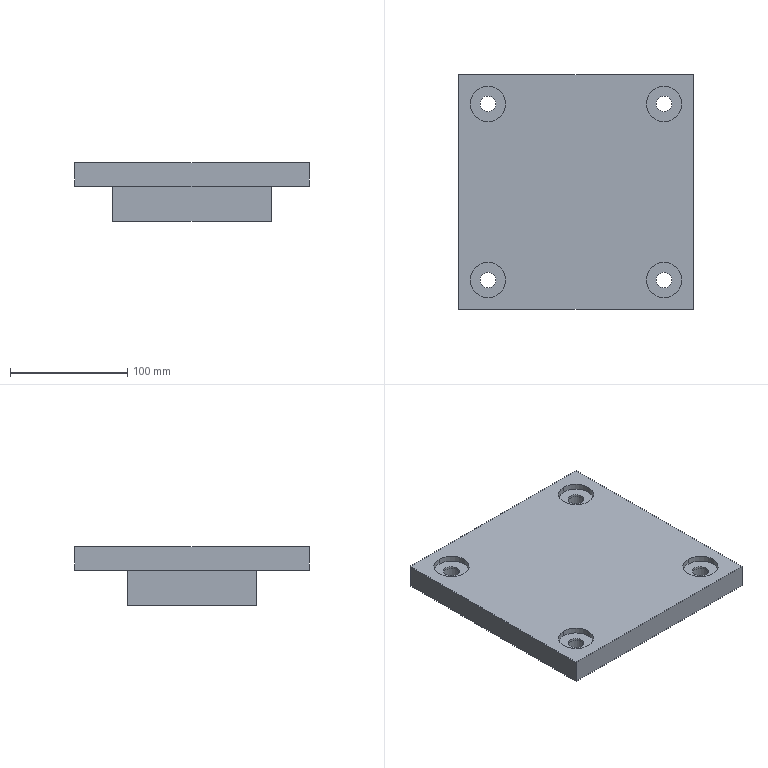Part | SolidWorks | features BaseBody 1 | 1 solid | 43 faces | box 200 x 200 x 50 mm | volume 1213881 mm3 | cylinder 24 | plane 19 | commonest cylinder face diameters 13.5 x8 20 x8 30 x8
STEP:
#1=CARTESIAN_POINT('',(65.,75.,18.));
#2=VERTEX_POINT('',#1);
#3=CARTESIAN_POINT('',(85.,75.,18.));
#4=VERTEX_POINT('',#3);
#5=CARTESIAN_POINT('',(75.,75.,18.));
#6=DIRECTION('',(0.,0.,1.));
#7=DIRECTION('',(-1.,0.,0.));
#8=AXIS2_PLACEMENT_3D('',#5,#6,#7);
#9=CIRCLE('',#8,10.);
#10=EDGE_CURVE('',#2,#4,#9,.T.);
#11=ORIENTED_EDGE('',*,*,#10,.T.);
#12=CARTESIAN_POINT('',(85.,75.,5.));
#13=VERTEX_POINT('',#12);
#14=CARTESIAN_POINT('',(85.,75.,18.));
#15=DIRECTION('',(0.,0.,-1.));
#16=VECTOR('',#15,1000.);
#17=LINE('',#14,#16);
#18=EDGE_CURVE('',#4,#13,#17,.T.);
#19=ORIENTED_EDGE('',*,*,#18,.T.);
#20=CARTESIAN_POINT('',(65.,75.,5.));
#21=VERTEX_POINT('',#20);
#22=CARTESIAN_POINT('',(75.,75.,5.));
#23=DIRECTION('',(0.,0.,-1.));
#24=DIRECTION('',(-1.,0.,0.));
#25=AXIS2_PLACEMENT_3D('',#22,#23,#24);
#26=CIRCLE('',#25,10.);
#27=EDGE_CURVE('',#13,#21,#26,.T.);
#28=ORIENTED_EDGE('',*,*,#27,.T.);
#29=CARTESIAN_POINT('',(65.,75.,18.));
#30=DIRECTION('',(0.,0.,-1.));
#31=VECTOR('',#30,1000.);
#32=LINE('',#29,#31);
#33=EDGE_CURVE('',#2,#21,#32,.T.);
#34=ORIENTED_EDGE('',*,*,#33,.F.);
#35=EDGE_LOOP('',(#11,#19,#28,#34));
#36=FACE_OUTER_BOUND('',#35,.T.);
#37=CARTESIAN_POINT('',(75.,75.,18.));
#38=DIRECTION('',(0.,0.,-1.));
#39=DIRECTION('',(-1.,0.,0.));
#40=AXIS2_PLACEMENT_3D('',#37,#38,#39);
#41=CYLINDRICAL_SURFACE('',#40,10.);
#42=ADVANCED_FACE('',(#36),#41,.F.);
#43=CARTESIAN_POINT('',(-85.,75.,18.));
#44=VERTEX_POINT('',#43);
#45=CARTESIAN_POINT('',(-65.,75.,18.));
#46=VERTEX_POINT('',#45);
#47=CARTESIAN_POINT('',(-75.,75.,18.));
#48=DIRECTION('',(0.,0.,1.));
#49=DIRECTION('',(-1.,0.,0.));
#50=AXIS2_PLACEMENT_3D('',#47,#48,#49);
#51=CIRCLE('',#50,10.);
#52=EDGE_CURVE('',#44,#46,#51,.T.);
#53=ORIENTED_EDGE('',*,*,#52,.T.);
#54=CARTESIAN_POINT('',(-65.,75.,5.));
#55=VERTEX_POINT('',#54);
#56=CARTESIAN_POINT('',(-65.,75.,18.));
#57=DIRECTION('',(0.,0.,-1.));
#58=VECTOR('',#57,1000.);
#59=LINE('',#56,#58);
#60=EDGE_CURVE('',#46,#55,#59,.T.);
#61=ORIENTED_EDGE('',*,*,#60,.T.);
#62=CARTESIAN_POINT('',(-85.,75.,5.));
#63=VERTEX_POINT('',#62);
#64=CARTESIAN_POINT('',(-75.,75.,5.));
#65=DIRECTION('',(0.,0.,1.));
#66=DIRECTION('',(-1.,0.,0.));
#67=AXIS2_PLACEMENT_3D('',#64,#65,#66);
#68=CIRCLE('',#67,10.);
#69=EDGE_CURVE('',#63,#55,#68,.T.);
#70=ORIENTED_EDGE('',*,*,#69,.F.);
#71=CARTESIAN_POINT('',(-85.,75.,18.));
#72=DIRECTION('',(0.,0.,-1.));
#73=VECTOR('',#72,1000.);
#74=LINE('',#71,#73);
#75=EDGE_CURVE('',#44,#63,#74,.T.);
#76=ORIENTED_EDGE('',*,*,#75,.F.);
#77=EDGE_LOOP('',(#53,#61,#70,#76));
#78=FACE_OUTER_BOUND('',#77,.T.);
#79=CARTESIAN_POINT('',(-75.,75.,18.));
#80=DIRECTION('',(0.,0.,-1.));
#81=DIRECTION('',(-1.,0.,0.));
#82=AXIS2_PLACEMENT_3D('',#79,#80,#81);
#83=CYLINDRICAL_SURFACE('',#82,10.);
#84=ADVANCED_FACE('',(#78),#83,.F.);
#85=CARTESIAN_POINT('',(-85.,-75.,18.));
#86=VERTEX_POINT('',#85);
#87=CARTESIAN_POINT('',(-65.,-75.,18.));
#88=VERTEX_POINT('',#87);
#89=CARTESIAN_POINT('',(-75.,-75.,18.));
#90=DIRECTION('',(0.,0.,1.));
#91=DIRECTION('',(-1.,0.,0.));
#92=AXIS2_PLACEMENT_3D('',#89,#90,#91);
#93=CIRCLE('',#92,10.);
#94=EDGE_CURVE('',#86,#88,#93,.T.);
#95=ORIENTED_EDGE('',*,*,#94,.T.);
#96=CARTESIAN_POINT('',(-65.,-75.,5.));
#97=VERTEX_POINT('',#96);
#98=CARTESIAN_POINT('',(-65.,-75.,18.));
#99=DIRECTION('',(0.,0.,-1.));
#100=VECTOR('',#99,1000.);
#101=LINE('',#98,#100);
#102=EDGE_CURVE('',#88,#97,#101,.T.);
#103=ORIENTED_EDGE('',*,*,#102,.T.);
#104=CARTESIAN_POINT('',(-85.,-75.,5.));
#105=VERTEX_POINT('',#104);
#106=CARTESIAN_POINT('',(-75.,-75.,5.));
#107=DIRECTION('',(0.,0.,1.));
#108=DIRECTION('',(-1.,0.,0.));
#109=AXIS2_PLACEMENT_3D('',#106,#107,#108);
#110=CIRCLE('',#109,10.);
#111=EDGE_CURVE('',#105,#97,#110,.T.);
#112=ORIENTED_EDGE('',*,*,#111,.F.);
#113=CARTESIAN_POINT('',(-85.,-75.,18.));
#114=DIRECTION('',(0.,0.,-1.));
#115=VECTOR('',#114,1000.);
#116=LINE('',#113,#115);
#117=EDGE_CURVE('',#86,#105,#116,.T.);
#118=ORIENTED_EDGE('',*,*,#117,.F.);
#119=EDGE_LOOP('',(#95,#103,#112,#118));
#120=FACE_OUTER_BOUND('',#119,.T.);
#121=CARTESIAN_POINT('',(-75.,-75.,18.));
#122=DIRECTION('',(0.,0.,-1.));
#123=DIRECTION('',(-1.,0.,0.));
#124=AXIS2_PLACEMENT_3D('',#121,#122,#123);
#125=CYLINDRICAL_SURFACE('',#124,10.);
#126=ADVANCED_FACE('',(#120),#125,.F.);
#127=CARTESIAN_POINT('',(65.,-75.,18.));
#128=VERTEX_POINT('',#127);
#129=CARTESIAN_POINT('',(85.,-75.,18.));
#130=VERTEX_POINT('',#129);
#131=CARTESIAN_POINT('',(75.,-75.,18.));
#132=DIRECTION('',(0.,0.,1.));
#133=DIRECTION('',(-1.,0.,0.));
#134=AXIS2_PLACEMENT_3D('',#131,#132,#133);
#135=CIRCLE('',#134,10.);
#136=EDGE_CURVE('',#128,#130,#135,.T.);
#137=ORIENTED_EDGE('',*,*,#136,.T.);
#138=CARTESIAN_POINT('',(85.,-75.,5.));
#139=VERTEX_POINT('',#138);
#140=CARTESIAN_POINT('',(85.,-75.,18.));
#141=DIRECTION('',(0.,0.,-1.));
#142=VECTOR('',#141,1000.);
#143=LINE('',#140,#142);
#144=EDGE_CURVE('',#130,#139,#143,.T.);
#145=ORIENTED_EDGE('',*,*,#144,.T.);
#146=CARTESIAN_POINT('',(65.,-75.,5.));
#147=VERTEX_POINT('',#146);
#148=CARTESIAN_POINT('',(75.,-75.,5.));
#149=DIRECTION('',(0.,0.,1.));
#150=DIRECTION('',(-1.,0.,0.));
#151=AXIS2_PLACEMENT_3D('',#148,#149,#150);
#152=CIRCLE('',#151,10.);
#153=EDGE_CURVE('',#147,#139,#152,.T.);
#154=ORIENTED_EDGE('',*,*,#153,.F.);
#155=CARTESIAN_POINT('',(65.,-75.,18.));
#156=DIRECTION('',(0.,0.,-1.));
#157=VECTOR('',#156,1000.);
#158=LINE('',#155,#157);
#159=EDGE_CURVE('',#128,#147,#158,.T.);
#160=ORIENTED_EDGE('',*,*,#159,.F.);
#161=EDGE_LOOP('',(#137,#145,#154,#160));
#162=FACE_OUTER_BOUND('',#161,.T.);
#163=CARTESIAN_POINT('',(75.,-75.,18.));
#164=DIRECTION('',(0.,0.,-1.));
#165=DIRECTION('',(-1.,0.,0.));
#166=AXIS2_PLACEMENT_3D('',#163,#164,#165);
#167=CYLINDRICAL_SURFACE('',#166,10.);
#168=ADVANCED_FACE('',(#162),#167,.F.);
#169=CARTESIAN_POINT('',(75.,81.75,20.));
#170=VERTEX_POINT('',#169);
#171=CARTESIAN_POINT('',(75.,68.25,20.));
#172=VERTEX_POINT('',#171);
#173=CARTESIAN_POINT('',(75.,75.,20.));
#174=DIRECTION('',(0.,0.,1.));
#175=DIRECTION('',(0.,1.,0.));
#176=AXIS2_PLACEMENT_3D('',#173,#174,#175);
#177=CIRCLE('',#176,6.75);
#178=EDGE_CURVE('',#170,#172,#177,.T.);
#179=ORIENTED_EDGE('',*,*,#178,.T.);
#180=CARTESIAN_POINT('',(75.,68.25,18.));
#181=VERTEX_POINT('',#180);
#182=CARTESIAN_POINT('',(75.,68.25,20.));
#183=DIRECTION('',(0.,0.,-1.));
#184=VECTOR('',#183,1000.);
#185=LINE('',#182,#184);
#186=EDGE_CURVE('',#172,#181,#185,.T.);
#187=ORIENTED_EDGE('',*,*,#186,.T.);
#188=CARTESIAN_POINT('',(75.,81.75,18.));
#189=VERTEX_POINT('',#188);
#190=CARTESIAN_POINT('',(75.,75.,18.));
#191=DIRECTION('',(0.,0.,-1.));
#192=DIRECTION('',(0.,1.,0.));
#193=AXIS2_PLACEMENT_3D('',#190,#191,#192);
#194=CIRCLE('',#193,6.75);
#195=EDGE_CURVE('',#181,#189,#194,.T.);
#196=ORIENTED_EDGE('',*,*,#195,.T.);
#197=CARTESIAN_POINT('',(75.,81.75,20.));
#198=DIRECTION('',(0.,0.,-1.));
#199=VECTOR('',#198,1000.);
#200=LINE('',#197,#199);
#201=EDGE_CURVE('',#170,#189,#200,.T.);
#202=ORIENTED_EDGE('',*,*,#201,.F.);
#203=EDGE_LOOP('',(#179,#187,#196,#202));
#204=FACE_OUTER_BOUND('',#203,.T.);
#205=CARTESIAN_POINT('',(75.,75.,20.));
#206=DIRECTION('',(0.,0.,-1.));
#207=DIRECTION('',(0.,1.,0.));
#208=AXIS2_PLACEMENT_3D('',#205,#206,#207);
#209=CYLINDRICAL_SURFACE('',#208,6.75);
#210=ADVANCED_FACE('',(#204),#209,.F.);
#211=CARTESIAN_POINT('',(-75.,81.75,20.));
#212=VERTEX_POINT('',#211);
#213=CARTESIAN_POINT('',(-75.,68.25,20.));
#214=VERTEX_POINT('',#213);
#215=CARTESIAN_POINT('',(-75.,75.,20.));
#216=DIRECTION('',(0.,0.,1.));
#217=DIRECTION('',(0.,1.,0.));
#218=AXIS2_PLACEMENT_3D('',#215,#216,#217);
#219=CIRCLE('',#218,6.75);
#220=EDGE_CURVE('',#212,#214,#219,.T.);
#221=ORIENTED_EDGE('',*,*,#220,.T.);
#222=CARTESIAN_POINT('',(-75.,68.25,18.));
#223=VERTEX_POINT('',#222);
#224=CARTESIAN_POINT('',(-75.,68.25,20.));
#225=DIRECTION('',(0.,0.,-1.));
#226=VECTOR('',#225,1000.);
#227=LINE('',#224,#226);
#228=EDGE_CURVE('',#214,#223,#227,.T.);
#229=ORIENTED_EDGE('',*,*,#228,.T.);
#230=CARTESIAN_POINT('',(-75.,81.75,18.));
#231=VERTEX_POINT('',#230);
#232=CARTESIAN_POINT('',(-75.,75.,18.));
#233=DIRECTION('',(0.,0.,-1.));
#234=DIRECTION('',(0.,1.,0.));
#235=AXIS2_PLACEMENT_3D('',#232,#233,#234);
#236=CIRCLE('',#235,6.75);
#237=EDGE_CURVE('',#223,#231,#236,.T.);
#238=ORIENTED_EDGE('',*,*,#237,.T.);
#239=CARTESIAN_POINT('',(-75.,81.75,20.));
#240=DIRECTION('',(0.,0.,-1.));
#241=VECTOR('',#240,1000.);
#242=LINE('',#239,#241);
#243=EDGE_CURVE('',#212,#231,#242,.T.);
#244=ORIENTED_EDGE('',*,*,#243,.F.);
#245=EDGE_LOOP('',(#221,#229,#238,#244));
#246=FACE_OUTER_BOUND('',#245,.T.);
#247=CARTESIAN_POINT('',(-75.,75.,20.));
#248=DIRECTION('',(0.,0.,-1.));
#249=DIRECTION('',(0.,1.,0.));
#250=AXIS2_PLACEMENT_3D('',#247,#248,#249);
#251=CYLINDRICAL_SURFACE('',#250,6.75);
#252=ADVANCED_FACE('',(#246),#251,.F.);
#253=CARTESIAN_POINT('',(-75.,-68.25,20.));
#254=VERTEX_POINT('',#253);
#255=CARTESIAN_POINT('',(-75.,-81.75,20.));
#256=VERTEX_POINT('',#255);
#257=CARTESIAN_POINT('',(-75.,-75.,20.));
#258=DIRECTION('',(0.,0.,1.));
#259=DIRECTION('',(0.,1.,0.));
#260=AXIS2_PLACEMENT_3D('',#257,#258,#259);
#261=CIRCLE('',#260,6.75);
#262=EDGE_CURVE('',#254,#256,#261,.T.);
#263=ORIENTED_EDGE('',*,*,#262,.T.);
#264=CARTESIAN_POINT('',(-75.,-81.75,18.));
#265=VERTEX_POINT('',#264);
#266=CARTESIAN_POINT('',(-75.,-81.75,20.));
#267=DIRECTION('',(0.,0.,-1.));
#268=VECTOR('',#267,1000.);
#269=LINE('',#266,#268);
#270=EDGE_CURVE('',#256,#265,#269,.T.);
#271=ORIENTED_EDGE('',*,*,#270,.T.);
#272=CARTESIAN_POINT('',(-75.,-68.25,18.));
#273=VERTEX_POINT('',#272);
#274=CARTESIAN_POINT('',(-75.,-75.,18.));
#275=DIRECTION('',(0.,0.,-1.));
#276=DIRECTION('',(0.,1.,0.));
#277=AXIS2_PLACEMENT_3D('',#274,#275,#276);
#278=CIRCLE('',#277,6.75);
#279=EDGE_CURVE('',#265,#273,#278,.T.);
#280=ORIENTED_EDGE('',*,*,#279,.T.);
#281=CARTESIAN_POINT('',(-75.,-68.25,20.));
#282=DIRECTION('',(0.,0.,-1.));
#283=VECTOR('',#282,1000.);
#284=LINE('',#281,#283);
#285=EDGE_CURVE('',#254,#273,#284,.T.);
#286=ORIENTED_EDGE('',*,*,#285,.F.);
#287=EDGE_LOOP('',(#263,#271,#280,#286));
#288=FACE_OUTER_BOUND('',#287,.T.);
#289=CARTESIAN_POINT('',(-75.,-75.,20.));
#290=DIRECTION('',(0.,0.,-1.));
#291=DIRECTION('',(0.,1.,0.));
#292=AXIS2_PLACEMENT_3D('',#289,#290,#291);
#293=CYLINDRICAL_SURFACE('',#292,6.75);
#294=ADVANCED_FACE('',(#288),#293,.F.);
#295=CARTESIAN_POINT('',(75.,-68.25,20.));
#296=VERTEX_POINT('',#295);
#297=CARTESIAN_POINT('',(75.,-81.75,20.));
#298=VERTEX_POINT('',#297);
#299=CARTESIAN_POINT('',(75.,-75.,20.));
#300=DIRECTION('',(0.,0.,1.));
#301=DIRECTION('',(0.,1.,0.));
#302=AXIS2_PLACEMENT_3D('',#299,#300,#301);
#303=CIRCLE('',#302,6.75);
#304=EDGE_CURVE('',#296,#298,#303,.T.);
#305=ORIENTED_EDGE('',*,*,#304,.T.);
#306=CARTESIAN_POINT('',(75.,-81.75,18.));
#307=VERTEX_POINT('',#306);
#308=CARTESIAN_POINT('',(75.,-81.75,20.));
#309=DIRECTION('',(0.,0.,-1.));
#310=VECTOR('',#309,1000.);
#311=LINE('',#308,#310);
#312=EDGE_CURVE('',#298,#307,#311,.T.);
#313=ORIENTED_EDGE('',*,*,#312,.T.);
#314=CARTESIAN_POINT('',(75.,-68.25,18.));
#315=VERTEX_POINT('',#314);
#316=CARTESIAN_POINT('',(75.,-75.,18.));
#317=DIRECTION('',(0.,0.,-1.));
#318=DIRECTION('',(0.,1.,0.));
#319=AXIS2_PLACEMENT_3D('',#316,#317,#318);
#320=CIRCLE('',#319,6.75);
#321=EDGE_CURVE('',#307,#315,#320,.T.);
#322=ORIENTED_EDGE('',*,*,#321,.T.);
#323=CARTESIAN_POINT('',(75.,-68.25,20.));
#324=DIRECTION('',(0.,0.,-1.));
#325=VECTOR('',#324,1000.);
#326=LINE('',#323,#325);
#327=EDGE_CURVE('',#296,#315,#326,.T.);
#328=ORIENTED_EDGE('',*,*,#327,.F.);
#329=EDGE_LOOP('',(#305,#313,#322,#328));
#330=FACE_OUTER_BOUND('',#329,.T.);
#331=CARTESIAN_POINT('',(75.,-75.,20.));
#332=DIRECTION('',(0.,0.,-1.));
#333=DIRECTION('',(0.,1.,0.));
#334=AXIS2_PLACEMENT_3D('',#331,#332,#333);
#335=CYLINDRICAL_SURFACE('',#334,6.75);
#336=ADVANCED_FACE('',(#330),#335,.F.);
#337=CARTESIAN_POINT('',(-75.,60.,20.));
#338=VERTEX_POINT('',#337);
#339=CARTESIAN_POINT('',(-75.,90.,20.));
#340=VERTEX_POINT('',#339);
#341=CARTESIAN_POINT('',(-75.,75.,20.));
#342=DIRECTION('',(0.,0.,-1.));
#343=DIRECTION('',(0.,-1.,0.));
#344=AXIS2_PLACEMENT_3D('',#341,#342,#343);
#345=CIRCLE('',#344,15.);
#346=EDGE_CURVE('',#338,#340,#345,.T.);
#347=ORIENTED_EDGE('',*,*,#346,.T.);
#348=CARTESIAN_POINT('',(-75.,90.,25.));
#349=VERTEX_POINT('',#348);
#350=CARTESIAN_POINT('',(-75.,90.,20.));
#351=DIRECTION('',(0.,0.,1.));
#352=VECTOR('',#351,1000.);
#353=LINE('',#350,#352);
#354=EDGE_CURVE('',#340,#349,#353,.T.);
#355=ORIENTED_EDGE('',*,*,#354,.T.);
#356=CARTESIAN_POINT('',(-75.,60.,25.));
#357=VERTEX_POINT('',#356);
#358=CARTESIAN_POINT('',(-75.,75.,25.));
#359=DIRECTION('',(0.,0.,1.));
#360=DIRECTION('',(0.,-1.,0.));
#361=AXIS2_PLACEMENT_3D('',#358,#359,#360);
#362=CIRCLE('',#361,15.);
#363=EDGE_CURVE('',#349,#357,#362,.T.);
#364=ORIENTED_EDGE('',*,*,#363,.T.);
#365=CARTESIAN_POINT('',(-75.,60.,20.));
#366=DIRECTION('',(0.,0.,1.));
#367=VECTOR('',#366,1000.);
#368=LINE('',#365,#367);
#369=EDGE_CURVE('',#338,#357,#368,.T.);
#370=ORIENTED_EDGE('',*,*,#369,.F.);
#371=EDGE_LOOP('',(#347,#355,#364,#370));
#372=FACE_OUTER_BOUND('',#371,.T.);
#373=CARTESIAN_POINT('',(-75.,75.,20.));
#374=DIRECTION('',(0.,0.,1.));
#375=DIRECTION('',(0.,-1.,0.));
#376=AXIS2_PLACEMENT_3D('',#373,#374,#375);
#377=CYLINDRICAL_SURFACE('',#376,15.);
#378=ADVANCED_FACE('',(#372),#377,.F.);
#379=CARTESIAN_POINT('',(-75.,-90.,20.));
#380=VERTEX_POINT('',#379);
#381=CARTESIAN_POINT('',(-75.,-60.,20.));
#382=VERTEX_POINT('',#381);
#383=CARTESIAN_POINT('',(-75.,-75.,20.));
#384=DIRECTION('',(0.,0.,-1.));
#385=DIRECTION('',(0.,-1.,0.));
#386=AXIS2_PLACEMENT_3D('',#383,#384,#385);
#387=CIRCLE('',#386,15.);
#388=EDGE_CURVE('',#380,#382,#387,.T.);
#389=ORIENTED_EDGE('',*,*,#388,.T.);
#390=CARTESIAN_POINT('',(-75.,-60.,25.));
#391=VERTEX_POINT('',#390);
#392=CARTESIAN_POINT('',(-75.,-60.,20.));
#393=DIRECTION('',(0.,0.,1.));
#394=VECTOR('',#393,1000.);
#395=LINE('',#392,#394);
#396=EDGE_CURVE('',#382,#391,#395,.T.);
#397=ORIENTED_EDGE('',*,*,#396,.T.);
#398=CARTESIAN_POINT('',(-75.,-90.,25.));
#399=VERTEX_POINT('',#398);
#400=CARTESIAN_POINT('',(-75.,-75.,25.));
#401=DIRECTION('',(0.,0.,1.));
#402=DIRECTION('',(0.,-1.,0.));
#403=AXIS2_PLACEMENT_3D('',#400,#401,#402);
#404=CIRCLE('',#403,15.);
#405=EDGE_CURVE('',#391,#399,#404,.T.);
#406=ORIENTED_EDGE('',*,*,#405,.T.);
#407=CARTESIAN_POINT('',(-75.,-90.,20.));
#408=DIRECTION('',(0.,0.,1.));
#409=VECTOR('',#408,1000.);
#410=LINE('',#407,#409);
#411=EDGE_CURVE('',#380,#399,#410,.T.);
#412=ORIENTED_EDGE('',*,*,#411,.F.);
#413=EDGE_LOOP('',(#389,#397,#406,#412));
#414=FACE_OUTER_BOUND('',#413,.T.);
#415=CARTESIAN_POINT('',(-75.,-75.,20.));
#416=DIRECTION('',(0.,0.,1.));
#417=DIRECTION('',(0.,-1.,0.));
#418=AXIS2_PLACEMENT_3D('',#415,#416,#417);
#419=CYLINDRICAL_SURFACE('',#418,15.);
#420=ADVANCED_FACE('',(#414),#419,.F.);
#421=CARTESIAN_POINT('',(75.,-90.,20.));
#422=VERTEX_POINT('',#421);
#423=CARTESIAN_POINT('',(75.,-60.,20.));
#424=VERTEX_POINT('',#423);
#425=CARTESIAN_POINT('',(75.,-75.,20.));
#426=DIRECTION('',(0.,0.,-1.));
#427=DIRECTION('',(0.,-1.,0.));
#428=AXIS2_PLACEMENT_3D('',#425,#426,#427);
#429=CIRCLE('',#428,15.);
#430=EDGE_CURVE('',#422,#424,#429,.T.);
#431=ORIENTED_EDGE('',*,*,#430,.T.);
#432=CARTESIAN_POINT('',(75.,-60.,25.));
#433=VERTEX_POINT('',#432);
#434=CARTESIAN_POINT('',(75.,-60.,20.));
#435=DIRECTION('',(0.,0.,1.));
#436=VECTOR('',#435,1000.);
#437=LINE('',#434,#436);
#438=EDGE_CURVE('',#424,#433,#437,.T.);
#439=ORIENTED_EDGE('',*,*,#438,.T.);
#440=CARTESIAN_POINT('',(75.,-90.,25.));
#441=VERTEX_POINT('',#440);
#442=CARTESIAN_POINT('',(75.,-75.,25.));
#443=DIRECTION('',(0.,0.,1.));
#444=DIRECTION('',(0.,-1.,0.));
#445=AXIS2_PLACEMENT_3D('',#442,#443,#444);
#446=CIRCLE('',#445,15.);
#447=EDGE_CURVE('',#433,#441,#446,.T.);
#448=ORIENTED_EDGE('',*,*,#447,.T.);
#449=CARTESIAN_POINT('',(75.,-90.,20.));
#450=DIRECTION('',(0.,0.,1.));
#451=VECTOR('',#450,1000.);
#452=LINE('',#449,#451);
#453=EDGE_CURVE('',#422,#441,#452,.T.);
#454=ORIENTED_EDGE('',*,*,#453,.F.);
#455=EDGE_LOOP('',(#431,#439,#448,#454));
#456=FACE_OUTER_BOUND('',#455,.T.);
#457=CARTESIAN_POINT('',(75.,-75.,20.));
#458=DIRECTION('',(0.,0.,1.));
#459=DIRECTION('',(0.,-1.,0.));
#460=AXIS2_PLACEMENT_3D('',#457,#458,#459);
#461=CYLINDRICAL_SURFACE('',#460,15.);
#462=ADVANCED_FACE('',(#456),#461,.F.);
#463=CARTESIAN_POINT('',(75.,60.,20.));
#464=VERTEX_POINT('',#463);
#465=CARTESIAN_POINT('',(75.,90.,20.));
#466=VERTEX_POINT('',#465);
#467=CARTESIAN_POINT('',(75.,75.,20.));
#468=DIRECTION('',(0.,0.,-1.));
#469=DIRECTION('',(0.,-1.,0.));
#470=AXIS2_PLACEMENT_3D('',#467,#468,#469);
#471=CIRCLE('',#470,15.);
#472=EDGE_CURVE('',#464,#466,#471,.T.);
#473=ORIENTED_EDGE('',*,*,#472,.T.);
#474=CARTESIAN_POINT('',(75.,90.,25.));
#475=VERTEX_POINT('',#474);
#476=CARTESIAN_POINT('',(75.,90.,20.));
#477=DIRECTION('',(0.,0.,1.));
#478=VECTOR('',#477,1000.);
#479=LINE('',#476,#478);
#480=EDGE_CURVE('',#466,#475,#479,.T.);
#481=ORIENTED_EDGE('',*,*,#480,.T.);
#482=CARTESIAN_POINT('',(75.,60.,25.));
#483=VERTEX_POINT('',#482);
#484=CARTESIAN_POINT('',(75.,75.,25.));
#485=DIRECTION('',(0.,0.,1.));
#486=DIRECTION('',(0.,-1.,0.));
#487=AXIS2_PLACEMENT_3D('',#484,#485,#486);
#488=CIRCLE('',#487,15.);
#489=EDGE_CURVE('',#475,#483,#488,.T.);
#490=ORIENTED_EDGE('',*,*,#489,.T.);
#491=CARTESIAN_POINT('',(75.,60.,20.));
#492=DIRECTION('',(0.,0.,1.));
#493=VECTOR('',#492,1000.);
#494=LINE('',#491,#493);
#495=EDGE_CURVE('',#464,#483,#494,.T.);
#496=ORIENTED_EDGE('',*,*,#495,.F.);
#497=EDGE_LOOP('',(#473,#481,#490,#496));
#498=FACE_OUTER_BOUND('',#497,.T.);
#499=CARTESIAN_POINT('',(75.,75.,20.));
#500=DIRECTION('',(0.,0.,1.));
#501=DIRECTION('',(0.,-1.,0.));
#502=AXIS2_PLACEMENT_3D('',#499,#500,#501);
#503=CYLINDRICAL_SURFACE('',#502,15.);
#504=ADVANCED_FACE('',(#498),#503,.F.);
#505=ORIENTED_EDGE('',*,*,#18,.F.);
#506=CARTESIAN_POINT('',(75.,75.,18.));
#507=DIRECTION('',(0.,0.,1.));
#508=DIRECTION('',(-1.,0.,0.));
#509=AXIS2_PLACEMENT_3D('',#506,#507,#508);
#510=CIRCLE('',#509,10.);
#511=EDGE_CURVE('',#4,#2,#510,.T.);
#512=ORIENTED_EDGE('',*,*,#511,.T.);
#513=ORIENTED_EDGE('',*,*,#33,.T.);
#514=CARTESIAN_POINT('',(75.,75.,5.));
#515=DIRECTION('',(0.,0.,-1.));
#516=DIRECTION('',(-1.,0.,0.));
#517=AXIS2_PLACEMENT_3D('',#514,#515,#516);
#518=CIRCLE('',#517,10.);
#519=EDGE_CURVE('',#21,#13,#518,.T.);
#520=ORIENTED_EDGE('',*,*,#519,.T.);
#521=EDGE_LOOP('',(#505,#512,#513,#520));
#522=FACE_OUTER_BOUND('',#521,.T.);
#523=CARTESIAN_POINT('',(75.,75.,18.));
#524=DIRECTION('',(0.,0.,-1.));
#525=DIRECTION('',(-1.,0.,0.));
#526=AXIS2_PLACEMENT_3D('',#523,#524,#525);
#527=CYLINDRICAL_SURFACE('',#526,10.);
#528=ADVANCED_FACE('',(#522),#527,.F.);
#529=CARTESIAN_POINT('',(-67.5,-55.,5.));
#530=VERTEX_POINT('',#529);
#531=CARTESIAN_POINT('',(67.5,-55.,5.));
#532=VERTEX_POINT('',#531);
#533=CARTESIAN_POINT('',(0.,-55.,5.));
#534=DIRECTION('',(1.,0.,0.));
#535=VECTOR('',#534,1000.);
#536=LINE('',#533,#535);
#537=EDGE_CURVE('',#530,#532,#536,.T.);
#538=ORIENTED_EDGE('',*,*,#537,.T.);
#539=CARTESIAN_POINT('',(67.5,55.,5.));
#540=VERTEX_POINT('',#539);
#541=CARTESIAN_POINT('',(67.5,0.,5.));
#542=DIRECTION('',(0.,1.,0.));
#543=VECTOR('',#542,1000.);
#544=LINE('',#541,#543);
#545=EDGE_CURVE('',#532,#540,#544,.T.);
#546=ORIENTED_EDGE('',*,*,#545,.T.);
#547=CARTESIAN_POINT('',(-67.5,55.,5.));
#548=VERTEX_POINT('',#547);
#549=CARTESIAN_POINT('',(0.,55.,5.));
#550=DIRECTION('',(-1.,0.,0.));
#551=VECTOR('',#550,1000.);
#552=LINE('',#549,#551);
#553=EDGE_CURVE('',#540,#548,#552,.T.);
#554=ORIENTED_EDGE('',*,*,#553,.T.);
#555=CARTESIAN_POINT('',(-67.5,0.,5.));
#556=DIRECTION('',(0.,-1.,0.));
#557=VECTOR('',#556,1000.);
#558=LINE('',#555,#557);
#559=EDGE_CURVE('',#548,#530,#558,.T.);
#560=ORIENTED_EDGE('',*,*,#559,.T.);
#561=EDGE_LOOP('',(#538,#546,#554,#560));
#562=FACE_BOUND('',#561,.T.);
#563=ORIENTED_EDGE('',*,*,#69,.T.);
#564=CARTESIAN_POINT('',(-75.,75.,5.));
#565=DIRECTION('',(0.,0.,1.));
#566=DIRECTION('',(-1.,0.,0.));
#567=AXIS2_PLACEMENT_3D('',#564,#565,#566);
#568=CIRCLE('',#567,10.);
#569=EDGE_CURVE('',#55,#63,#568,.T.);
#570=ORIENTED_EDGE('',*,*,#569,.T.);
#571=EDGE_LOOP('',(#563,#570));
#572=FACE_BOUND('',#571,.T.);
#573=ORIENTED_EDGE('',*,*,#111,.T.);
#574=CARTESIAN_POINT('',(-75.,-75.,5.));
#575=DIRECTION('',(0.,0.,1.));
#576=DIRECTION('',(-1.,0.,0.));
#577=AXIS2_PLACEMENT_3D('',#574,#575,#576);
#578=CIRCLE('',#577,10.);
#579=EDGE_CURVE('',#97,#105,#578,.T.);
#580=ORIENTED_EDGE('',*,*,#579,.T.);
#581=EDGE_LOOP('',(#573,#580));
#582=FACE_BOUND('',#581,.T.);
#583=ORIENTED_EDGE('',*,*,#153,.T.);
#584=CARTESIAN_POINT('',(75.,-75.,5.));
#585=DIRECTION('',(0.,0.,1.));
#586=DIRECTION('',(-1.,0.,0.));
#587=AXIS2_PLACEMENT_3D('',#584,#585,#586);
#588=CIRCLE('',#587,10.);
#589=EDGE_CURVE('',#139,#147,#588,.T.);
#590=ORIENTED_EDGE('',*,*,#589,.T.);
#591=EDGE_LOOP('',(#583,#590));
#592=FACE_BOUND('',#591,.T.);
#593=ORIENTED_EDGE('',*,*,#519,.F.);
#594=ORIENTED_EDGE('',*,*,#27,.F.);
#595=EDGE_LOOP('',(#593,#594));
#596=FACE_BOUND('',#595,.T.);
#597=CARTESIAN_POINT('',(-100.,-100.,5.));
#598=VERTEX_POINT('',#597);
#599=CARTESIAN_POINT('',(-100.,100.,5.));
#600=VERTEX_POINT('',#599);
#601=CARTESIAN_POINT('',(-100.,0.,5.));
#602=DIRECTION('',(0.,1.,0.));
#603=VECTOR('',#602,1000.);
#604=LINE('',#601,#603);
#605=EDGE_CURVE('',#598,#600,#604,.T.);
#606=ORIENTED_EDGE('',*,*,#605,.T.);
#607=CARTESIAN_POINT('',(100.,100.,5.));
#608=VERTEX_POINT('',#607);
#609=CARTESIAN_POINT('',(0.,100.,5.));
#610=DIRECTION('',(1.,0.,0.));
#611=VECTOR('',#610,1000.);
#612=LINE('',#609,#611);
#613=EDGE_CURVE('',#600,#608,#612,.T.);
#614=ORIENTED_EDGE('',*,*,#613,.T.);
#615=CARTESIAN_POINT('',(100.,-100.,5.));
#616=VERTEX_POINT('',#615);
#617=CARTESIAN_POINT('',(100.,0.,5.));
#618=DIRECTION('',(0.,-1.,0.));
#619=VECTOR('',#618,1000.);
#620=LINE('',#617,#619);
#621=EDGE_CURVE('',#608,#616,#620,.T.);
#622=ORIENTED_EDGE('',*,*,#621,.T.);
#623=CARTESIAN_POINT('',(0.,-100.,5.));
#624=DIRECTION('',(-1.,0.,0.));
#625=VECTOR('',#624,1000.);
#626=LINE('',#623,#625);
#627=EDGE_CURVE('',#616,#598,#626,.T.);
#628=ORIENTED_EDGE('',*,*,#627,.T.);
#629=EDGE_LOOP('',(#606,#614,#622,#628));
#630=FACE_OUTER_BOUND('',#629,.T.);
#631=CARTESIAN_POINT('',(100.,-100.,5.));
#632=DIRECTION('',(0.,0.,-1.));
#633=DIRECTION('',(-1.,0.,0.));
#634=AXIS2_PLACEMENT_3D('',#631,#632,#633);
#635=PLANE('',#634);
#636=ADVANCED_FACE('',(#562,#572,#582,#592,#596,#630),#635,.T.);
#637=CARTESIAN_POINT('',(75.,75.,18.));
#638=DIRECTION('',(0.,0.,-1.));
#639=DIRECTION('',(0.,1.,0.));
#640=AXIS2_PLACEMENT_3D('',#637,#638,#639);
#641=CIRCLE('',#640,6.75);
#642=EDGE_CURVE('',#189,#181,#641,.T.);
#643=ORIENTED_EDGE('',*,*,#642,.F.);
#644=ORIENTED_EDGE('',*,*,#195,.F.);
#645=EDGE_LOOP('',(#643,#644));
#646=FACE_BOUND('',#645,.T.);
#647=ORIENTED_EDGE('',*,*,#10,.F.);
#648=ORIENTED_EDGE('',*,*,#511,.F.);
#649=EDGE_LOOP('',(#647,#648));
#650=FACE_OUTER_BOUND('',#649,.T.);
#651=CARTESIAN_POINT('',(64.88,64.88,18.));
#652=DIRECTION('',(0.,0.,1.));
#653=DIRECTION('',(1.,0.,0.));
#654=AXIS2_PLACEMENT_3D('',#651,#652,#653);
#655=PLANE('',#654);
#656=ADVANCED_FACE('',(#646,#650),#655,.F.);
#657=ORIENTED_EDGE('',*,*,#545,.F.);
#658=CARTESIAN_POINT('',(67.5,-55.,-25.));
#659=VERTEX_POINT('',#658);
#660=CARTESIAN_POINT('',(67.5,-55.,-10.));
#661=DIRECTION('',(0.,0.,-1.));
#662=VECTOR('',#661,1000.);
#663=LINE('',#660,#662);
#664=EDGE_CURVE('',#532,#659,#663,.T.);
#665=ORIENTED_EDGE('',*,*,#664,.T.);
#666=CARTESIAN_POINT('',(67.5,55.,-25.));
#667=VERTEX_POINT('',#666);
#668=CARTESIAN_POINT('',(67.5,0.,-25.));
#669=DIRECTION('',(0.,1.,0.));
#670=VECTOR('',#669,1000.);
#671=LINE('',#668,#670);
#672=EDGE_CURVE('',#659,#667,#671,.T.);
#673=ORIENTED_EDGE('',*,*,#672,.T.);
#674=CARTESIAN_POINT('',(67.5,55.,-10.));
#675=DIRECTION('',(0.,0.,1.));
#676=VECTOR('',#675,1000.);
#677=LINE('',#674,#676);
#678=EDGE_CURVE('',#667,#540,#677,.T.);
#679=ORIENTED_EDGE('',*,*,#678,.T.);
#680=EDGE_LOOP('',(#657,#665,#673,#679));
#681=FACE_OUTER_BOUND('',#680,.T.);
#682=CARTESIAN_POINT('',(67.5,-55.,5.));
#683=DIRECTION('',(1.,0.,0.));
#684=DIRECTION('',(0.,0.,-1.));
#685=AXIS2_PLACEMENT_3D('',#682,#683,#684);
#686=PLANE('',#685);
#687=ADVANCED_FACE('',(#681),#686,.T.);
#688=ORIENTED_EDGE('',*,*,#537,.F.);
#689=CARTESIAN_POINT('',(-67.5,-55.,-25.));
#690=VERTEX_POINT('',#689);
#691=CARTESIAN_POINT('',(-67.5,-55.,-10.));
#692=DIRECTION('',(0.,0.,-1.));
#693=VECTOR('',#692,1000.);
#694=LINE('',#691,#693);
#695=EDGE_CURVE('',#530,#690,#694,.T.);
#696=ORIENTED_EDGE('',*,*,#695,.T.);
#697=CARTESIAN_POINT('',(0.,-55.,-25.));
#698=DIRECTION('',(1.,0.,0.));
#699=VECTOR('',#698,1000.);
#700=LINE('',#697,#699);
#701=EDGE_CURVE('',#690,#659,#700,.T.);
#702=ORIENTED_EDGE('',*,*,#701,.T.);
#703=ORIENTED_EDGE('',*,*,#664,.F.);
#704=EDGE_LOOP('',(#688,#696,#702,#703));
#705=FACE_OUTER_BOUND('',#704,.T.);
#706=CARTESIAN_POINT('',(-67.5,-55.,-25.));
#707=DIRECTION('',(0.,-1.,0.));
#708=DIRECTION('',(1.,0.,0.));
#709=AXIS2_PLACEMENT_3D('',#706,#707,#708);
#710=PLANE('',#709);
#711=ADVANCED_FACE('',(#705),#710,.T.);
#712=ORIENTED_EDGE('',*,*,#559,.F.);
#713=CARTESIAN_POINT('',(-67.5,55.,-25.));
#714=VERTEX_POINT('',#713);
#715=CARTESIAN_POINT('',(-67.5,55.,-10.));
#716=DIRECTION('',(0.,0.,-1.));
#717=VECTOR('',#716,1000.);
#718=LINE('',#715,#717);
#719=EDGE_CURVE('',#548,#714,#718,.T.);
#720=ORIENTED_EDGE('',*,*,#719,.T.);
#721=CARTESIAN_POINT('',(-67.5,0.,-25.));
#722=DIRECTION('',(0.,-1.,0.));
#723=VECTOR('',#722,1000.);
#724=LINE('',#721,#723);
#725=EDGE_CURVE('',#714,#690,#724,.T.);
#726=ORIENTED_EDGE('',*,*,#725,.T.);
#727=ORIENTED_EDGE('',*,*,#695,.F.);
#728=EDGE_LOOP('',(#712,#720,#726,#727));
#729=FACE_OUTER_BOUND('',#728,.T.);
#730=CARTESIAN_POINT('',(-67.5,-55.,-25.));
#731=DIRECTION('',(-1.,0.,0.));
#732=DIRECTION('',(0.,0.,1.));
#733=AXIS2_PLACEMENT_3D('',#730,#731,#732);
#734=PLANE('',#733);
#735=ADVANCED_FACE('',(#729),#734,.T.);
#736=ORIENTED_EDGE('',*,*,#553,.F.);
#737=ORIENTED_EDGE('',*,*,#678,.F.);
#738=CARTESIAN_POINT('',(0.,55.,-25.));
#739=DIRECTION('',(-1.,0.,0.));
#740=VECTOR('',#739,1000.);
#741=LINE('',#738,#740);
#742=EDGE_CURVE('',#667,#714,#741,.T.);
#743=ORIENTED_EDGE('',*,*,#742,.T.);
#744=ORIENTED_EDGE('',*,*,#719,.F.);
#745=EDGE_LOOP('',(#736,#737,#743,#744));
#746=FACE_OUTER_BOUND('',#745,.T.);
#747=CARTESIAN_POINT('',(67.5,55.,-25.));
#748=DIRECTION('',(0.,1.,0.));
#749=DIRECTION('',(-1.,0.,0.));
#750=AXIS2_PLACEMENT_3D('',#747,#748,#749);
#751=PLANE('',#750);
#752=ADVANCED_FACE('',(#746),#751,.T.);
#753=ORIENTED_EDGE('',*,*,#60,.F.);
#754=CARTESIAN_POINT('',(-75.,75.,18.));
#755=DIRECTION('',(0.,0.,1.));
#756=DIRECTION('',(-1.,0.,0.));
#757=AXIS2_PLACEMENT_3D('',#754,#755,#756);
#758=CIRCLE('',#757,10.);
#759=EDGE_CURVE('',#46,#44,#758,.T.);
#760=ORIENTED_EDGE('',*,*,#759,.T.);
#761=ORIENTED_EDGE('',*,*,#75,.T.);
#762=ORIENTED_EDGE('',*,*,#569,.F.);
#763=EDGE_LOOP('',(#753,#760,#761,#762));
#764=FACE_OUTER_BOUND('',#763,.T.);
#765=CARTESIAN_POINT('',(-75.,75.,18.));
#766=DIRECTION('',(0.,0.,-1.));
#767=DIRECTION('',(-1.,0.,0.));
#768=AXIS2_PLACEMENT_3D('',#765,#766,#767);
#769=CYLINDRICAL_SURFACE('',#768,10.);
#770=ADVANCED_FACE('',(#764),#769,.F.);
#771=ORIENTED_EDGE('',*,*,#102,.F.);
#772=CARTESIAN_POINT('',(-75.,-75.,18.));
#773=DIRECTION('',(0.,0.,1.));
#774=DIRECTION('',(-1.,0.,0.));
#775=AXIS2_PLACEMENT_3D('',#772,#773,#774);
#776=CIRCLE('',#775,10.);
#777=EDGE_CURVE('',#88,#86,#776,.T.);
#778=ORIENTED_EDGE('',*,*,#777,.T.);
#779=ORIENTED_EDGE('',*,*,#117,.T.);
#780=ORIENTED_EDGE('',*,*,#579,.F.);
#781=EDGE_LOOP('',(#771,#778,#779,#780));
#782=FACE_OUTER_BOUND('',#781,.T.);
#783=CARTESIAN_POINT('',(-75.,-75.,18.));
#784=DIRECTION('',(0.,0.,-1.));
#785=DIRECTION('',(-1.,0.,0.));
#786=AXIS2_PLACEMENT_3D('',#783,#784,#785);
#787=CYLINDRICAL_SURFACE('',#786,10.);
#788=ADVANCED_FACE('',(#782),#787,.F.);
#789=ORIENTED_EDGE('',*,*,#144,.F.);
#790=CARTESIAN_POINT('',(75.,-75.,18.));
#791=DIRECTION('',(0.,0.,1.));
#792=DIRECTION('',(-1.,0.,0.));
#793=AXIS2_PLACEMENT_3D('',#790,#791,#792);
#794=CIRCLE('',#793,10.);
#795=EDGE_CURVE('',#130,#128,#794,.T.);
#796=ORIENTED_EDGE('',*,*,#795,.T.);
#797=ORIENTED_EDGE('',*,*,#159,.T.);
#798=ORIENTED_EDGE('',*,*,#589,.F.);
#799=EDGE_LOOP('',(#789,#796,#797,#798));
#800=FACE_OUTER_BOUND('',#799,.T.);
#801=CARTESIAN_POINT('',(75.,-75.,18.));
#802=DIRECTION('',(0.,0.,-1.));
#803=DIRECTION('',(-1.,0.,0.));
#804=AXIS2_PLACEMENT_3D('',#801,#802,#803);
#805=CYLINDRICAL_SURFACE('',#804,10.);
#806=ADVANCED_FACE('',(#800),#805,.F.);
#807=CARTESIAN_POINT('',(-100.,100.,25.));
#808=VERTEX_POINT('',#807);
#809=CARTESIAN_POINT('',(-100.,100.,15.));
#810=DIRECTION('',(0.,0.,-1.));
#811=VECTOR('',#810,1000.);
#812=LINE('',#809,#811);
#813=EDGE_CURVE('',#808,#600,#812,.T.);
#814=ORIENTED_EDGE('',*,*,#813,.F.);
#815=CARTESIAN_POINT('',(100.,100.,25.));
#816=VERTEX_POINT('',#815);
#817=CARTESIAN_POINT('',(0.,100.,25.));
#818=DIRECTION('',(-1.,0.,0.));
#819=VECTOR('',#818,1000.);
#820=LINE('',#817,#819);
#821=EDGE_CURVE('',#816,#808,#820,.T.);
#822=ORIENTED_EDGE('',*,*,#821,.F.);
#823=CARTESIAN_POINT('',(100.,100.,15.));
#824=DIRECTION('',(0.,0.,1.));
#825=VECTOR('',#824,1000.);
#826=LINE('',#823,#825);
#827=EDGE_CURVE('',#608,#816,#826,.T.);
#828=ORIENTED_EDGE('',*,*,#827,.F.);
#829=ORIENTED_EDGE('',*,*,#613,.F.);
#830=EDGE_LOOP('',(#814,#822,#828,#829));
#831=FACE_OUTER_BOUND('',#830,.T.);
#832=CARTESIAN_POINT('',(-100.,100.,25.));
#833=DIRECTION('',(0.,-1.,0.));
#834=DIRECTION('',(0.,0.,-1.));
#835=AXIS2_PLACEMENT_3D('',#832,#833,#834);
#836=PLANE('',#835);
#837=ADVANCED_FACE('',(#831),#836,.F.);
#838=CARTESIAN_POINT('',(-100.,-100.,25.));
#839=VERTEX_POINT('',#838);
#840=CARTESIAN_POINT('',(-100.,-100.,15.));
#841=DIRECTION('',(0.,0.,-1.));
#842=VECTOR('',#841,1000.);
#843=LINE('',#840,#842);
#844=EDGE_CURVE('',#839,#598,#843,.T.);
#845=ORIENTED_EDGE('',*,*,#844,.F.);
#846=CARTESIAN_POINT('',(-100.,0.,25.));
#847=DIRECTION('',(0.,-1.,0.));
#848=VECTOR('',#847,1000.);
#849=LINE('',#846,#848);
#850=EDGE_CURVE('',#808,#839,#849,.T.);
#851=ORIENTED_EDGE('',*,*,#850,.F.);
#852=ORIENTED_EDGE('',*,*,#813,.T.);
#853=ORIENTED_EDGE('',*,*,#605,.F.);
#854=EDGE_LOOP('',(#845,#851,#852,#853));
#855=FACE_OUTER_BOUND('',#854,.T.);
#856=CARTESIAN_POINT('',(-100.,-100.,25.));
#857=DIRECTION('',(1.,0.,0.));
#858=DIRECTION('',(0.,0.,-1.));
#859=AXIS2_PLACEMENT_3D('',#856,#857,#858);
#860=PLANE('',#859);
#861=ADVANCED_FACE('',(#855),#860,.F.);
#862=CARTESIAN_POINT('',(100.,-100.,25.));
#863=VERTEX_POINT('',#862);
#864=CARTESIAN_POINT('',(100.,-100.,15.));
#865=DIRECTION('',(0.,0.,-1.));
#866=VECTOR('',#865,1000.);
#867=LINE('',#864,#866);
#868=EDGE_CURVE('',#863,#616,#867,.T.);
#869=ORIENTED_EDGE('',*,*,#868,.F.);
#870=CARTESIAN_POINT('',(0.,-100.,25.));
#871=DIRECTION('',(1.,0.,0.));
#872=VECTOR('',#871,1000.);
#873=LINE('',#870,#872);
#874=EDGE_CURVE('',#839,#863,#873,.T.);
#875=ORIENTED_EDGE('',*,*,#874,.F.);
#876=ORIENTED_EDGE('',*,*,#844,.T.);
#877=ORIENTED_EDGE('',*,*,#627,.F.);
#878=EDGE_LOOP('',(#869,#875,#876,#877));
#879=FACE_OUTER_BOUND('',#878,.T.);
#880=CARTESIAN_POINT('',(-100.,-100.,5.));
#881=DIRECTION('',(0.,1.,0.));
#882=DIRECTION('',(0.,0.,1.));
#883=AXIS2_PLACEMENT_3D('',#880,#881,#882);
#884=PLANE('',#883);
#885=ADVANCED_FACE('',(#879),#884,.F.);
#886=ORIENTED_EDGE('',*,*,#827,.T.);
#887=CARTESIAN_POINT('',(100.,0.,25.));
#888=DIRECTION('',(0.,1.,0.));
#889=VECTOR('',#888,1000.);
#890=LINE('',#887,#889);
#891=EDGE_CURVE('',#863,#816,#890,.T.);
#892=ORIENTED_EDGE('',*,*,#891,.F.);
#893=ORIENTED_EDGE('',*,*,#868,.T.);
#894=ORIENTED_EDGE('',*,*,#621,.F.);
#895=EDGE_LOOP('',(#886,#892,#893,#894));
#896=FACE_OUTER_BOUND('',#895,.T.);
#897=CARTESIAN_POINT('',(100.,-100.,5.));
#898=DIRECTION('',(-1.,0.,0.));
#899=DIRECTION('',(0.,0.,1.));
#900=AXIS2_PLACEMENT_3D('',#897,#898,#899);
#901=PLANE('',#900);
#902=ADVANCED_FACE('',(#896),#901,.F.);
#903=ORIENTED_EDGE('',*,*,#186,.F.);
#904=CARTESIAN_POINT('',(75.,75.,20.));
#905=DIRECTION('',(0.,0.,1.));
#906=DIRECTION('',(0.,1.,0.));
#907=AXIS2_PLACEMENT_3D('',#904,#905,#906);
#908=CIRCLE('',#907,6.75);
#909=EDGE_CURVE('',#172,#170,#908,.T.);
#910=ORIENTED_EDGE('',*,*,#909,.T.);
#911=ORIENTED_EDGE('',*,*,#201,.T.);
#912=ORIENTED_EDGE('',*,*,#642,.T.);
#913=EDGE_LOOP('',(#903,#910,#911,#912));
#914=FACE_OUTER_BOUND('',#913,.T.);
#915=CARTESIAN_POINT('',(75.,75.,20.));
#916=DIRECTION('',(0.,0.,-1.));
#917=DIRECTION('',(0.,1.,0.));
#918=AXIS2_PLACEMENT_3D('',#915,#916,#917);
#919=CYLINDRICAL_SURFACE('',#918,6.75);
#920=ADVANCED_FACE('',(#914),#919,.F.);
#921=ORIENTED_EDGE('',*,*,#701,.F.);
#922=ORIENTED_EDGE('',*,*,#725,.F.);
#923=ORIENTED_EDGE('',*,*,#742,.F.);
#924=ORIENTED_EDGE('',*,*,#672,.F.);
#925=EDGE_LOOP('',(#921,#922,#923,#924));
#926=FACE_OUTER_BOUND('',#925,.T.);
#927=CARTESIAN_POINT('',(67.5,-55.,-25.));
#928=DIRECTION('',(0.,0.,-1.));
#929=DIRECTION('',(-1.,0.,0.));
#930=AXIS2_PLACEMENT_3D('',#927,#928,#929);
#931=PLANE('',#930);
#932=ADVANCED_FACE('',(#926),#931,.T.);
#933=CARTESIAN_POINT('',(-75.,75.,18.));
#934=DIRECTION('',(0.,0.,-1.));
#935=DIRECTION('',(0.,1.,0.));
#936=AXIS2_PLACEMENT_3D('',#933,#934,#935);
#937=CIRCLE('',#936,6.75);
#938=EDGE_CURVE('',#231,#223,#937,.T.);
#939=ORIENTED_EDGE('',*,*,#938,.F.);
#940=ORIENTED_EDGE('',*,*,#237,.F.);
#941=EDGE_LOOP('',(#939,#940));
#942=FACE_BOUND('',#941,.T.);
#943=ORIENTED_EDGE('',*,*,#52,.F.);
#944=ORIENTED_EDGE('',*,*,#759,.F.);
#945=EDGE_LOOP('',(#943,#944));
#946=FACE_OUTER_BOUND('',#945,.T.);
#947=CARTESIAN_POINT('',(-85.12,64.88,18.));
#948=DIRECTION('',(0.,0.,1.));
#949=DIRECTION('',(1.,0.,0.));
#950=AXIS2_PLACEMENT_3D('',#947,#948,#949);
#951=PLANE('',#950);
#952=ADVANCED_FACE('',(#942,#946),#951,.F.);
#953=CARTESIAN_POINT('',(-75.,-75.,18.));
#954=DIRECTION('',(0.,0.,-1.));
#955=DIRECTION('',(0.,1.,0.));
#956=AXIS2_PLACEMENT_3D('',#953,#954,#955);
#957=CIRCLE('',#956,6.75);
#958=EDGE_CURVE('',#273,#265,#957,.T.);
#959=ORIENTED_EDGE('',*,*,#958,.F.);
#960=ORIENTED_EDGE('',*,*,#279,.F.);
#961=EDGE_LOOP('',(#959,#960));
#962=FACE_BOUND('',#961,.T.);
#963=ORIENTED_EDGE('',*,*,#94,.F.);
#964=ORIENTED_EDGE('',*,*,#777,.F.);
#965=EDGE_LOOP('',(#963,#964));
#966=FACE_OUTER_BOUND('',#965,.T.);
#967=CARTESIAN_POINT('',(-85.12,-85.12,18.));
#968=DIRECTION('',(0.,0.,1.));
#969=DIRECTION('',(1.,0.,0.));
#970=AXIS2_PLACEMENT_3D('',#967,#968,#969);
#971=PLANE('',#970);
#972=ADVANCED_FACE('',(#962,#966),#971,.F.);
#973=CARTESIAN_POINT('',(75.,-75.,18.));
#974=DIRECTION('',(0.,0.,-1.));
#975=DIRECTION('',(0.,1.,0.));
#976=AXIS2_PLACEMENT_3D('',#973,#974,#975);
#977=CIRCLE('',#976,6.75);
#978=EDGE_CURVE('',#315,#307,#977,.T.);
#979=ORIENTED_EDGE('',*,*,#978,.F.);
#980=ORIENTED_EDGE('',*,*,#321,.F.);
#981=EDGE_LOOP('',(#979,#980));
#982=FACE_BOUND('',#981,.T.);
#983=ORIENTED_EDGE('',*,*,#136,.F.);
#984=ORIENTED_EDGE('',*,*,#795,.F.);
#985=EDGE_LOOP('',(#983,#984));
#986=FACE_OUTER_BOUND('',#985,.T.);
#987=CARTESIAN_POINT('',(64.88,-85.12,18.));
#988=DIRECTION('',(0.,0.,1.));
#989=DIRECTION('',(1.,0.,0.));
#990=AXIS2_PLACEMENT_3D('',#987,#988,#989);
#991=PLANE('',#990);
#992=ADVANCED_FACE('',(#982,#986),#991,.F.);
#993=CARTESIAN_POINT('',(-75.,75.,25.));
#994=DIRECTION('',(0.,0.,1.));
#995=DIRECTION('',(0.,-1.,0.));
#996=AXIS2_PLACEMENT_3D('',#993,#994,#995);
#997=CIRCLE('',#996,15.);
#998=EDGE_CURVE('',#357,#349,#997,.T.);
#999=ORIENTED_EDGE('',*,*,#998,.F.);
#1000=ORIENTED_EDGE('',*,*,#363,.F.);
#1001=EDGE_LOOP('',(#999,#1000));
#1002=FACE_BOUND('',#1001,.T.);
#1003=CARTESIAN_POINT('',(-75.,-75.,25.));
#1004=DIRECTION('',(0.,0.,1.));
#1005=DIRECTION('',(0.,-1.,0.));
#1006=AXIS2_PLACEMENT_3D('',#1003,#1004,#1005);
#1007=CIRCLE('',#1006,15.);
#1008=EDGE_CURVE('',#399,#391,#1007,.T.);
#1009=ORIENTED_EDGE('',*,*,#1008,.F.);
#1010=ORIENTED_EDGE('',*,*,#405,.F.);
#1011=EDGE_LOOP('',(#1009,#1010));
#1012=FACE_BOUND('',#1011,.T.);
#1013=CARTESIAN_POINT('',(75.,-75.,25.));
#1014=DIRECTION('',(0.,0.,1.));
#1015=DIRECTION('',(0.,-1.,0.));
#1016=AXIS2_PLACEMENT_3D('',#1013,#1014,#1015);
#1017=CIRCLE('',#1016,15.);
#1018=EDGE_CURVE('',#441,#433,#1017,.T.);
#1019=ORIENTED_EDGE('',*,*,#1018,.F.);
#1020=ORIENTED_EDGE('',*,*,#447,.F.);
#1021=EDGE_LOOP('',(#1019,#1020));
#1022=FACE_BOUND('',#1021,.T.);
#1023=CARTESIAN_POINT('',(75.,75.,25.));
#1024=DIRECTION('',(0.,0.,1.));
#1025=DIRECTION('',(0.,-1.,0.));
#1026=AXIS2_PLACEMENT_3D('',#1023,#1024,#1025);
#1027=CIRCLE('',#1026,15.);
#1028=EDGE_CURVE('',#483,#475,#1027,.T.);
#1029=ORIENTED_EDGE('',*,*,#1028,.F.);
#1030=ORIENTED_EDGE('',*,*,#489,.F.);
#1031=EDGE_LOOP('',(#1029,#1030));
#1032=FACE_BOUND('',#1031,.T.);
#1033=ORIENTED_EDGE('',*,*,#821,.T.);
#1034=ORIENTED_EDGE('',*,*,#850,.T.);
#1035=ORIENTED_EDGE('',*,*,#874,.T.);
#1036=ORIENTED_EDGE('',*,*,#891,.T.);
#1037=EDGE_LOOP('',(#1033,#1034,#1035,#1036));
#1038=FACE_OUTER_BOUND('',#1037,.T.);
#1039=CARTESIAN_POINT('',(100.,-100.,25.));
#1040=DIRECTION('',(0.,0.,-1.));
#1041=DIRECTION('',(-1.,0.,0.));
#1042=AXIS2_PLACEMENT_3D('',#1039,#1040,#1041);
#1043=PLANE('',#1042);
#1044=ADVANCED_FACE('',(#1002,#1012,#1022,#1032,#1038),#1043,.F.);
#1045=ORIENTED_EDGE('',*,*,#178,.F.);
#1046=ORIENTED_EDGE('',*,*,#909,.F.);
#1047=EDGE_LOOP('',(#1045,#1046));
#1048=FACE_BOUND('',#1047,.T.);
#1049=ORIENTED_EDGE('',*,*,#472,.F.);
#1050=CARTESIAN_POINT('',(75.,75.,20.));
#1051=DIRECTION('',(0.,0.,-1.));
#1052=DIRECTION('',(0.,-1.,0.));
#1053=AXIS2_PLACEMENT_3D('',#1050,#1051,#1052);
#1054=CIRCLE('',#1053,15.);
#1055=EDGE_CURVE('',#466,#464,#1054,.T.);
#1056=ORIENTED_EDGE('',*,*,#1055,.F.);
#1057=EDGE_LOOP('',(#1049,#1056));
#1058=FACE_OUTER_BOUND('',#1057,.T.);
#1059=CARTESIAN_POINT('',(90.18,59.82,20.));
#1060=DIRECTION('',(0.,0.,-1.));
#1061=DIRECTION('',(-1.,0.,0.));
#1062=AXIS2_PLACEMENT_3D('',#1059,#1060,#1061);
#1063=PLANE('',#1062);
#1064=ADVANCED_FACE('',(#1048,#1058),#1063,.F.);
#1065=ORIENTED_EDGE('',*,*,#228,.F.);
#1066=CARTESIAN_POINT('',(-75.,75.,20.));
#1067=DIRECTION('',(0.,0.,1.));
#1068=DIRECTION('',(0.,1.,0.));
#1069=AXIS2_PLACEMENT_3D('',#1066,#1067,#1068);
#1070=CIRCLE('',#1069,6.75);
#1071=EDGE_CURVE('',#214,#212,#1070,.T.);
#1072=ORIENTED_EDGE('',*,*,#1071,.T.);
#1073=ORIENTED_EDGE('',*,*,#243,.T.);
#1074=ORIENTED_EDGE('',*,*,#938,.T.);
#1075=EDGE_LOOP('',(#1065,#1072,#1073,#1074));
#1076=FACE_OUTER_BOUND('',#1075,.T.);
#1077=CARTESIAN_POINT('',(-75.,75.,20.));
#1078=DIRECTION('',(0.,0.,-1.));
#1079=DIRECTION('',(0.,1.,0.));
#1080=AXIS2_PLACEMENT_3D('',#1077,#1078,#1079);
#1081=CYLINDRICAL_SURFACE('',#1080,6.75);
#1082=ADVANCED_FACE('',(#1076),#1081,.F.);
#1083=ORIENTED_EDGE('',*,*,#270,.F.);
#1084=CARTESIAN_POINT('',(-75.,-75.,20.));
#1085=DIRECTION('',(0.,0.,1.));
#1086=DIRECTION('',(0.,1.,0.));
#1087=AXIS2_PLACEMENT_3D('',#1084,#1085,#1086);
#1088=CIRCLE('',#1087,6.75);
#1089=EDGE_CURVE('',#256,#254,#1088,.T.);
#1090=ORIENTED_EDGE('',*,*,#1089,.T.);
#1091=ORIENTED_EDGE('',*,*,#285,.T.);
#1092=ORIENTED_EDGE('',*,*,#958,.T.);
#1093=EDGE_LOOP('',(#1083,#1090,#1091,#1092));
#1094=FACE_OUTER_BOUND('',#1093,.T.);
#1095=CARTESIAN_POINT('',(-75.,-75.,20.));
#1096=DIRECTION('',(0.,0.,-1.));
#1097=DIRECTION('',(0.,1.,0.));
#1098=AXIS2_PLACEMENT_3D('',#1095,#1096,#1097);
#1099=CYLINDRICAL_SURFACE('',#1098,6.75);
#1100=ADVANCED_FACE('',(#1094),#1099,.F.);
#1101=ORIENTED_EDGE('',*,*,#312,.F.);
#1102=CARTESIAN_POINT('',(75.,-75.,20.));
#1103=DIRECTION('',(0.,0.,1.));
#1104=DIRECTION('',(0.,1.,0.));
#1105=AXIS2_PLACEMENT_3D('',#1102,#1103,#1104);
#1106=CIRCLE('',#1105,6.75);
#1107=EDGE_CURVE('',#298,#296,#1106,.T.);
#1108=ORIENTED_EDGE('',*,*,#1107,.T.);
#1109=ORIENTED_EDGE('',*,*,#327,.T.);
#1110=ORIENTED_EDGE('',*,*,#978,.T.);
#1111=EDGE_LOOP('',(#1101,#1108,#1109,#1110));
#1112=FACE_OUTER_BOUND('',#1111,.T.);
#1113=CARTESIAN_POINT('',(75.,-75.,20.));
#1114=DIRECTION('',(0.,0.,-1.));
#1115=DIRECTION('',(0.,1.,0.));
#1116=AXIS2_PLACEMENT_3D('',#1113,#1114,#1115);
#1117=CYLINDRICAL_SURFACE('',#1116,6.75);
#1118=ADVANCED_FACE('',(#1112),#1117,.F.);
#1119=ORIENTED_EDGE('',*,*,#354,.F.);
#1120=CARTESIAN_POINT('',(-75.,75.,20.));
#1121=DIRECTION('',(0.,0.,-1.));
#1122=DIRECTION('',(0.,-1.,0.));
#1123=AXIS2_PLACEMENT_3D('',#1120,#1121,#1122);
#1124=CIRCLE('',#1123,15.);
#1125=EDGE_CURVE('',#340,#338,#1124,.T.);
#1126=ORIENTED_EDGE('',*,*,#1125,.T.);
#1127=ORIENTED_EDGE('',*,*,#369,.T.);
#1128=ORIENTED_EDGE('',*,*,#998,.T.);
#1129=EDGE_LOOP('',(#1119,#1126,#1127,#1128));
#1130=FACE_OUTER_BOUND('',#1129,.T.);
#1131=CARTESIAN_POINT('',(-75.,75.,20.));
#1132=DIRECTION('',(0.,0.,1.));
#1133=DIRECTION('',(0.,-1.,0.));
#1134=AXIS2_PLACEMENT_3D('',#1131,#1132,#1133);
#1135=CYLINDRICAL_SURFACE('',#1134,15.);
#1136=ADVANCED_FACE('',(#1130),#1135,.F.);
#1137=ORIENTED_EDGE('',*,*,#396,.F.);
#1138=CARTESIAN_POINT('',(-75.,-75.,20.));
#1139=DIRECTION('',(0.,0.,-1.));
#1140=DIRECTION('',(0.,-1.,0.));
#1141=AXIS2_PLACEMENT_3D('',#1138,#1139,#1140);
#1142=CIRCLE('',#1141,15.);
#1143=EDGE_CURVE('',#382,#380,#1142,.T.);
#1144=ORIENTED_EDGE('',*,*,#1143,.T.);
#1145=ORIENTED_EDGE('',*,*,#411,.T.);
#1146=ORIENTED_EDGE('',*,*,#1008,.T.);
#1147=EDGE_LOOP('',(#1137,#1144,#1145,#1146));
#1148=FACE_OUTER_BOUND('',#1147,.T.);
#1149=CARTESIAN_POINT('',(-75.,-75.,20.));
#1150=DIRECTION('',(0.,0.,1.));
#1151=DIRECTION('',(0.,-1.,0.));
#1152=AXIS2_PLACEMENT_3D('',#1149,#1150,#1151);
#1153=CYLINDRICAL_SURFACE('',#1152,15.);
#1154=ADVANCED_FACE('',(#1148),#1153,.F.);
#1155=ORIENTED_EDGE('',*,*,#438,.F.);
#1156=CARTESIAN_POINT('',(75.,-75.,20.));
#1157=DIRECTION('',(0.,0.,-1.));
#1158=DIRECTION('',(0.,-1.,0.));
#1159=AXIS2_PLACEMENT_3D('',#1156,#1157,#1158);
#1160=CIRCLE('',#1159,15.);
#1161=EDGE_CURVE('',#424,#422,#1160,.T.);
#1162=ORIENTED_EDGE('',*,*,#1161,.T.);
#1163=ORIENTED_EDGE('',*,*,#453,.T.);
#1164=ORIENTED_EDGE('',*,*,#1018,.T.);
#1165=EDGE_LOOP('',(#1155,#1162,#1163,#1164));
#1166=FACE_OUTER_BOUND('',#1165,.T.);
#1167=CARTESIAN_POINT('',(75.,-75.,20.));
#1168=DIRECTION('',(0.,0.,1.));
#1169=DIRECTION('',(0.,-1.,0.));
#1170=AXIS2_PLACEMENT_3D('',#1167,#1168,#1169);
#1171=CYLINDRICAL_SURFACE('',#1170,15.);
#1172=ADVANCED_FACE('',(#1166),#1171,.F.);
#1173=ORIENTED_EDGE('',*,*,#480,.F.);
#1174=ORIENTED_EDGE('',*,*,#1055,.T.);
#1175=ORIENTED_EDGE('',*,*,#495,.T.);
#1176=ORIENTED_EDGE('',*,*,#1028,.T.);
#1177=EDGE_LOOP('',(#1173,#1174,#1175,#1176));
#1178=FACE_OUTER_BOUND('',#1177,.T.);
#1179=CARTESIAN_POINT('',(75.,75.,20.));
#1180=DIRECTION('',(0.,0.,1.));
#1181=DIRECTION('',(0.,-1.,0.));
#1182=AXIS2_PLACEMENT_3D('',#1179,#1180,#1181);
#1183=CYLINDRICAL_SURFACE('',#1182,15.);
#1184=ADVANCED_FACE('',(#1178),#1183,.F.);
#1185=ORIENTED_EDGE('',*,*,#220,.F.);
#1186=ORIENTED_EDGE('',*,*,#1071,.F.);
#1187=EDGE_LOOP('',(#1185,#1186));
#1188=FACE_BOUND('',#1187,.T.);
#1189=ORIENTED_EDGE('',*,*,#346,.F.);
#1190=ORIENTED_EDGE('',*,*,#1125,.F.);
#1191=EDGE_LOOP('',(#1189,#1190));
#1192=FACE_OUTER_BOUND('',#1191,.T.);
#1193=CARTESIAN_POINT('',(-90.18,59.82,20.));
#1194=DIRECTION('',(0.,0.,1.));
#1195=DIRECTION('',(1.,0.,0.));
#1196=AXIS2_PLACEMENT_3D('',#1193,#1194,#1195);
#1197=PLANE('',#1196);
#1198=ADVANCED_FACE('',(#1188,#1192),#1197,.T.);
#1199=ORIENTED_EDGE('',*,*,#262,.F.);
#1200=ORIENTED_EDGE('',*,*,#1089,.F.);
#1201=EDGE_LOOP('',(#1199,#1200));
#1202=FACE_BOUND('',#1201,.T.);
#1203=ORIENTED_EDGE('',*,*,#388,.F.);
#1204=ORIENTED_EDGE('',*,*,#1143,.F.);
#1205=EDGE_LOOP('',(#1203,#1204));
#1206=FACE_OUTER_BOUND('',#1205,.T.);
#1207=CARTESIAN_POINT('',(-59.82,-90.18,20.));
#1208=DIRECTION('',(0.,0.,-1.));
#1209=DIRECTION('',(-1.,0.,0.));
#1210=AXIS2_PLACEMENT_3D('',#1207,#1208,#1209);
#1211=PLANE('',#1210);
#1212=ADVANCED_FACE('',(#1202,#1206),#1211,.F.);
#1213=ORIENTED_EDGE('',*,*,#304,.F.);
#1214=ORIENTED_EDGE('',*,*,#1107,.F.);
#1215=EDGE_LOOP('',(#1213,#1214));
#1216=FACE_BOUND('',#1215,.T.);
#1217=ORIENTED_EDGE('',*,*,#430,.F.);
#1218=ORIENTED_EDGE('',*,*,#1161,.F.);
#1219=EDGE_LOOP('',(#1217,#1218));
#1220=FACE_OUTER_BOUND('',#1219,.T.);
#1221=CARTESIAN_POINT('',(59.82,-90.18,20.));
#1222=DIRECTION('',(0.,0.,1.));
#1223=DIRECTION('',(1.,0.,0.));
#1224=AXIS2_PLACEMENT_3D('',#1221,#1222,#1223);
#1225=PLANE('',#1224);
#1226=ADVANCED_FACE('',(#1216,#1220),#1225,.T.);
#1227=CLOSED_SHELL('',(#42,#84,#126,#168,#210,#252,#294,#336,#378,#420,#462,#504,#528,#636,#656,#687,#711,#735,#752,#770,#788,#806,#837,#861,#885,#902,#920,#932,#952,#972,#992,#1044,#1064,#1082,#1100,#1118,#1136,#1154,#1172,#1184,#1198,#1212,#1226));
#1228=MANIFOLD_SOLID_BREP('',#1227);
#1229=CARTESIAN_POINT('',(0.,0.,0.));
#1230=DIRECTION('',(0.,0.,1.));
#1231=DIRECTION('',(1.,0.,0.));
#1232=AXIS2_PLACEMENT_3D('',#1229,#1230,#1231);
#1233=(LENGTH_UNIT()NAMED_UNIT(*)SI_UNIT(.MILLI.,.METRE.));
#1234=UNCERTAINTY_MEASURE_WITH_UNIT(LENGTH_MEASURE(0.00001),#1233,'','');
#1235=(NAMED_UNIT(*)PLANE_ANGLE_UNIT()SI_UNIT($,.RADIAN.));
#1236=(NAMED_UNIT(*)SI_UNIT($,.STERADIAN.)SOLID_ANGLE_UNIT());
#1237=(GEOMETRIC_REPRESENTATION_CONTEXT(3)GLOBAL_UNCERTAINTY_ASSIGNED_CONTEXT((#1234))GLOBAL_UNIT_ASSIGNED_CONTEXT((#1233,#1235,#1236))REPRESENTATION_CONTEXT('',''));
#1238=ADVANCED_BREP_SHAPE_REPRESENTATION('',(#1228,#1232),#1237);